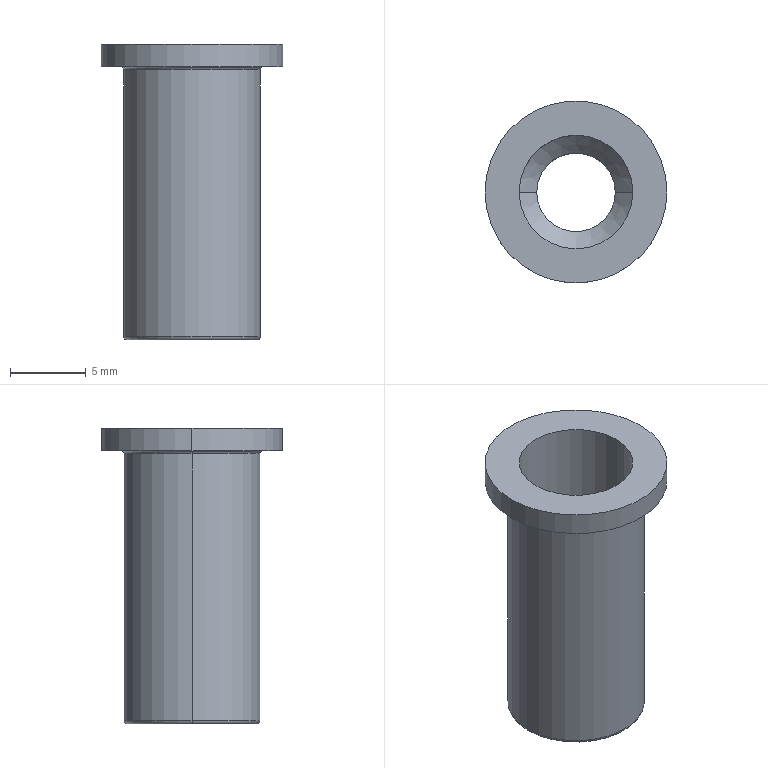Part | SolidWorks | features Chamfer 2, Cut 2, Boss 1, Extrusion 1, Fillet 1, LPattern 1, RevCut 1 | 1 solid | 19 faces | box 12 x 12 x 19.5 mm | volume 659.077 mm3 | cylinder 8 | cone 4 | torus 4 | plane 3 | commonest cylinder face diameters 5.188 x2 7.5 x2 9 x2 12 x2
STEP:
#1=CARTESIAN_POINT('',(2.594,0.,-19.241));
#2=VERTEX_POINT('',#1);
#3=CARTESIAN_POINT('',(-2.594,0.,-19.241));
#4=VERTEX_POINT('',#3);
#5=CARTESIAN_POINT('',(0.,0.,-19.241));
#6=DIRECTION('',(0.,0.,-1.));
#7=DIRECTION('',(-1.,0.,0.));
#8=AXIS2_PLACEMENT_3D('',#5,#6,#7);
#9=CIRCLE('',#8,2.594);
#10=EDGE_CURVE('',#2,#4,#9,.T.);
#11=ORIENTED_EDGE('',*,*,#10,.F.);
#12=CARTESIAN_POINT('',(2.853,0.,-19.5));
#13=VERTEX_POINT('',#12);
#14=CARTESIAN_POINT('',(2.853,0.,-19.5));
#15=DIRECTION('',(0.7071,0.,-0.7071));
#16=VECTOR('',#15,1000.);
#17=LINE('',#14,#16);
#18=EDGE_CURVE('',#2,#13,#17,.T.);
#19=ORIENTED_EDGE('',*,*,#18,.T.);
#20=CARTESIAN_POINT('',(-2.853,0.,-19.5));
#21=VERTEX_POINT('',#20);
#22=CARTESIAN_POINT('',(0.,0.,-19.5));
#23=DIRECTION('',(0.,0.,1.));
#24=DIRECTION('',(-1.,0.,0.));
#25=AXIS2_PLACEMENT_3D('',#22,#23,#24);
#26=CIRCLE('',#25,2.853);
#27=EDGE_CURVE('',#21,#13,#26,.T.);
#28=ORIENTED_EDGE('',*,*,#27,.F.);
#29=CARTESIAN_POINT('',(-2.853,0.,-19.5));
#30=DIRECTION('',(-0.7071,0.,-0.7071));
#31=VECTOR('',#30,1000.);
#32=LINE('',#29,#31);
#33=EDGE_CURVE('',#4,#21,#32,.T.);
#34=ORIENTED_EDGE('',*,*,#33,.F.);
#35=EDGE_LOOP('',(#11,#19,#28,#34));
#36=FACE_OUTER_BOUND('',#35,.T.);
#37=CARTESIAN_POINT('',(0.,0.,-19.5));
#38=DIRECTION('',(0.,0.,-1.));
#39=DIRECTION('',(-1.,0.,0.));
#40=AXIS2_PLACEMENT_3D('',#37,#38,#39);
#41=CONICAL_SURFACE('',#40,2.853,0.7854);
#42=ADVANCED_FACE('',(#36),#41,.F.);
#43=CARTESIAN_POINT('',(-2.594,0.,-11.156));
#44=VERTEX_POINT('',#43);
#45=CARTESIAN_POINT('',(2.594,0.,-11.156));
#46=VERTEX_POINT('',#45);
#47=CARTESIAN_POINT('',(0.,0.,-11.156));
#48=DIRECTION('',(0.,0.,1.));
#49=DIRECTION('',(1.,0.,0.));
#50=AXIS2_PLACEMENT_3D('',#47,#48,#49);
#51=CIRCLE('',#50,2.594);
#52=EDGE_CURVE('',#44,#46,#51,.T.);
#53=ORIENTED_EDGE('',*,*,#52,.F.);
#54=CARTESIAN_POINT('',(-3.75,0.,-10.));
#55=VERTEX_POINT('',#54);
#56=CARTESIAN_POINT('',(-2.594,0.,-11.156));
#57=DIRECTION('',(-0.7071,0.,0.7071));
#58=VECTOR('',#57,1000.);
#59=LINE('',#56,#58);
#60=EDGE_CURVE('',#44,#55,#59,.T.);
#61=ORIENTED_EDGE('',*,*,#60,.T.);
#62=CARTESIAN_POINT('',(3.75,0.,-10.));
#63=VERTEX_POINT('',#62);
#64=CARTESIAN_POINT('',(0.,0.,-10.));
#65=DIRECTION('',(0.,0.,1.));
#66=DIRECTION('',(1.,0.,0.));
#67=AXIS2_PLACEMENT_3D('',#64,#65,#66);
#68=CIRCLE('',#67,3.75);
#69=EDGE_CURVE('',#55,#63,#68,.T.);
#70=ORIENTED_EDGE('',*,*,#69,.T.);
#71=CARTESIAN_POINT('',(2.594,0.,-11.156));
#72=DIRECTION('',(0.7071,0.,0.7071));
#73=VECTOR('',#72,1000.);
#74=LINE('',#71,#73);
#75=EDGE_CURVE('',#46,#63,#74,.T.);
#76=ORIENTED_EDGE('',*,*,#75,.F.);
#77=EDGE_LOOP('',(#53,#61,#70,#76));
#78=FACE_OUTER_BOUND('',#77,.T.);
#79=CARTESIAN_POINT('',(0.,0.,-11.156));
#80=DIRECTION('',(0.,0.,1.));
#81=DIRECTION('',(1.,0.,0.));
#82=AXIS2_PLACEMENT_3D('',#79,#80,#81);
#83=CONICAL_SURFACE('',#82,2.594,0.7854);
#84=ADVANCED_FACE('',(#78),#83,.F.);
#85=CARTESIAN_POINT('',(-4.7,0.,-1.5));
#86=VERTEX_POINT('',#85);
#87=CARTESIAN_POINT('',(4.7,0.,-1.5));
#88=VERTEX_POINT('',#87);
#89=CARTESIAN_POINT('',(0.,0.,-1.5));
#90=DIRECTION('',(0.,0.,1.));
#91=DIRECTION('',(1.,0.,0.));
#92=AXIS2_PLACEMENT_3D('',#89,#90,#91);
#93=CIRCLE('',#92,4.7);
#94=EDGE_CURVE('',#86,#88,#93,.T.);
#95=ORIENTED_EDGE('',*,*,#94,.F.);
#96=CARTESIAN_POINT('',(-4.5,0.,-1.7));
#97=VERTEX_POINT('',#96);
#98=CARTESIAN_POINT('',(-4.7,0.,-1.7));
#99=DIRECTION('',(0.,1.,0.));
#100=DIRECTION('',(-1.,0.,0.));
#101=AXIS2_PLACEMENT_3D('',#98,#99,#100);
#102=CIRCLE('',#101,0.2);
#103=EDGE_CURVE('',#86,#97,#102,.T.);
#104=ORIENTED_EDGE('',*,*,#103,.T.);
#105=CARTESIAN_POINT('',(4.5,0.,-1.7));
#106=VERTEX_POINT('',#105);
#107=CARTESIAN_POINT('',(0.,0.,-1.7));
#108=DIRECTION('',(0.,0.,-1.));
#109=DIRECTION('',(1.,0.,0.));
#110=AXIS2_PLACEMENT_3D('',#107,#108,#109);
#111=CIRCLE('',#110,4.5);
#112=EDGE_CURVE('',#106,#97,#111,.T.);
#113=ORIENTED_EDGE('',*,*,#112,.F.);
#114=CARTESIAN_POINT('',(4.7,0.,-1.7));
#115=DIRECTION('',(0.,-1.,0.));
#116=DIRECTION('',(0.,0.,-1.));
#117=AXIS2_PLACEMENT_3D('',#114,#115,#116);
#118=CIRCLE('',#117,0.2);
#119=EDGE_CURVE('',#88,#106,#118,.T.);
#120=ORIENTED_EDGE('',*,*,#119,.F.);
#121=EDGE_LOOP('',(#95,#104,#113,#120));
#122=FACE_OUTER_BOUND('',#121,.T.);
#123=CARTESIAN_POINT('',(0.,0.,-1.7));
#124=DIRECTION('',(0.,0.,1.));
#125=DIRECTION('',(1.,0.,0.));
#126=AXIS2_PLACEMENT_3D('',#123,#124,#125);
#127=TOROIDAL_SURFACE('',#126,4.7,0.2);
#128=ADVANCED_FACE('',(#122),#127,.F.);
#129=CARTESIAN_POINT('',(4.5,0.,-19.3));
#130=VERTEX_POINT('',#129);
#131=CARTESIAN_POINT('',(-4.5,0.,-19.3));
#132=VERTEX_POINT('',#131);
#133=CARTESIAN_POINT('',(0.,0.,-19.3));
#134=DIRECTION('',(0.,0.,1.));
#135=DIRECTION('',(-1.,0.,0.));
#136=AXIS2_PLACEMENT_3D('',#133,#134,#135);
#137=CIRCLE('',#136,4.5);
#138=EDGE_CURVE('',#130,#132,#137,.T.);
#139=ORIENTED_EDGE('',*,*,#138,.F.);
#140=CARTESIAN_POINT('',(4.3,0.,-19.5));
#141=VERTEX_POINT('',#140);
#142=CARTESIAN_POINT('',(4.3,0.,-19.3));
#143=DIRECTION('',(0.,1.,0.));
#144=DIRECTION('',(-1.,0.,0.));
#145=AXIS2_PLACEMENT_3D('',#142,#143,#144);
#146=CIRCLE('',#145,0.2);
#147=EDGE_CURVE('',#130,#141,#146,.T.);
#148=ORIENTED_EDGE('',*,*,#147,.T.);
#149=CARTESIAN_POINT('',(-4.3,0.,-19.5));
#150=VERTEX_POINT('',#149);
#151=CARTESIAN_POINT('',(0.,0.,-19.5));
#152=DIRECTION('',(0.,0.,-1.));
#153=DIRECTION('',(-1.,0.,0.));
#154=AXIS2_PLACEMENT_3D('',#151,#152,#153);
#155=CIRCLE('',#154,4.3);
#156=EDGE_CURVE('',#150,#141,#155,.T.);
#157=ORIENTED_EDGE('',*,*,#156,.F.);
#158=CARTESIAN_POINT('',(-4.3,0.,-19.3));
#159=DIRECTION('',(0.,-1.,0.));
#160=DIRECTION('',(0.,0.,-1.));
#161=AXIS2_PLACEMENT_3D('',#158,#159,#160);
#162=CIRCLE('',#161,0.2);
#163=EDGE_CURVE('',#132,#150,#162,.T.);
#164=ORIENTED_EDGE('',*,*,#163,.F.);
#165=EDGE_LOOP('',(#139,#148,#157,#164));
#166=FACE_OUTER_BOUND('',#165,.T.);
#167=CARTESIAN_POINT('',(0.,0.,-19.3));
#168=DIRECTION('',(0.,0.,-1.));
#169=DIRECTION('',(-1.,0.,0.));
#170=AXIS2_PLACEMENT_3D('',#167,#168,#169);
#171=TOROIDAL_SURFACE('',#170,4.3,0.2);
#172=ADVANCED_FACE('',(#166),#171,.T.);
#173=ORIENTED_EDGE('',*,*,#10,.T.);
#174=CARTESIAN_POINT('',(-2.594,0.,-19.5));
#175=DIRECTION('',(0.,0.,1.));
#176=VECTOR('',#175,1000.);
#177=LINE('',#174,#176);
#178=EDGE_CURVE('',#4,#44,#177,.T.);
#179=ORIENTED_EDGE('',*,*,#178,.T.);
#180=ORIENTED_EDGE('',*,*,#52,.T.);
#181=CARTESIAN_POINT('',(2.594,0.,-19.5));
#182=DIRECTION('',(0.,0.,1.));
#183=VECTOR('',#182,1000.);
#184=LINE('',#181,#183);
#185=EDGE_CURVE('',#2,#46,#184,.T.);
#186=ORIENTED_EDGE('',*,*,#185,.F.);
#187=EDGE_LOOP('',(#173,#179,#180,#186));
#188=FACE_OUTER_BOUND('',#187,.T.);
#189=CARTESIAN_POINT('',(0.,0.,-19.5));
#190=DIRECTION('',(0.,0.,1.));
#191=DIRECTION('',(1.,0.,0.));
#192=AXIS2_PLACEMENT_3D('',#189,#190,#191);
#193=CYLINDRICAL_SURFACE('',#192,2.594);
#194=ADVANCED_FACE('',(#188),#193,.F.);
#195=ORIENTED_EDGE('',*,*,#69,.F.);
#196=CARTESIAN_POINT('',(-3.75,0.,0.));
#197=VERTEX_POINT('',#196);
#198=CARTESIAN_POINT('',(-3.75,0.,-10.));
#199=DIRECTION('',(0.,0.,1.));
#200=VECTOR('',#199,1000.);
#201=LINE('',#198,#200);
#202=EDGE_CURVE('',#55,#197,#201,.T.);
#203=ORIENTED_EDGE('',*,*,#202,.T.);
#204=CARTESIAN_POINT('',(3.75,0.,0.));
#205=VERTEX_POINT('',#204);
#206=CARTESIAN_POINT('',(0.,0.,0.));
#207=DIRECTION('',(0.,0.,1.));
#208=DIRECTION('',(1.,0.,0.));
#209=AXIS2_PLACEMENT_3D('',#206,#207,#208);
#210=CIRCLE('',#209,3.75);
#211=EDGE_CURVE('',#197,#205,#210,.T.);
#212=ORIENTED_EDGE('',*,*,#211,.T.);
#213=CARTESIAN_POINT('',(3.75,0.,-10.));
#214=DIRECTION('',(0.,0.,1.));
#215=VECTOR('',#214,1000.);
#216=LINE('',#213,#215);
#217=EDGE_CURVE('',#63,#205,#216,.T.);
#218=ORIENTED_EDGE('',*,*,#217,.F.);
#219=EDGE_LOOP('',(#195,#203,#212,#218));
#220=FACE_OUTER_BOUND('',#219,.T.);
#221=CARTESIAN_POINT('',(0.,0.,-10.));
#222=DIRECTION('',(0.,0.,1.));
#223=DIRECTION('',(1.,0.,0.));
#224=AXIS2_PLACEMENT_3D('',#221,#222,#223);
#225=CYLINDRICAL_SURFACE('',#224,3.75);
#226=ADVANCED_FACE('',(#220),#225,.F.);
#227=ORIENTED_EDGE('',*,*,#138,.T.);
#228=CARTESIAN_POINT('',(-4.5,0.,-19.5));
#229=DIRECTION('',(0.,0.,1.));
#230=VECTOR('',#229,1000.);
#231=LINE('',#228,#230);
#232=EDGE_CURVE('',#132,#97,#231,.T.);
#233=ORIENTED_EDGE('',*,*,#232,.T.);
#234=CARTESIAN_POINT('',(0.,0.,-1.7));
#235=DIRECTION('',(0.,0.,-1.));
#236=DIRECTION('',(1.,0.,0.));
#237=AXIS2_PLACEMENT_3D('',#234,#235,#236);
#238=CIRCLE('',#237,4.5);
#239=EDGE_CURVE('',#97,#106,#238,.T.);
#240=ORIENTED_EDGE('',*,*,#239,.T.);
#241=CARTESIAN_POINT('',(4.5,0.,-19.5));
#242=DIRECTION('',(0.,0.,1.));
#243=VECTOR('',#242,1000.);
#244=LINE('',#241,#243);
#245=EDGE_CURVE('',#130,#106,#244,.T.);
#246=ORIENTED_EDGE('',*,*,#245,.F.);
#247=EDGE_LOOP('',(#227,#233,#240,#246));
#248=FACE_OUTER_BOUND('',#247,.T.);
#249=CARTESIAN_POINT('',(0.,0.,-19.5));
#250=DIRECTION('',(0.,0.,1.));
#251=DIRECTION('',(1.,0.,0.));
#252=AXIS2_PLACEMENT_3D('',#249,#250,#251);
#253=CYLINDRICAL_SURFACE('',#252,4.5);
#254=ADVANCED_FACE('',(#248),#253,.T.);
#255=CARTESIAN_POINT('',(6.,0.,-1.5));
#256=VERTEX_POINT('',#255);
#257=CARTESIAN_POINT('',(-6.,0.,-1.5));
#258=VERTEX_POINT('',#257);
#259=CARTESIAN_POINT('',(0.,0.,-1.5));
#260=DIRECTION('',(0.,0.,1.));
#261=DIRECTION('',(1.,0.,0.));
#262=AXIS2_PLACEMENT_3D('',#259,#260,#261);
#263=CIRCLE('',#262,6.);
#264=EDGE_CURVE('',#256,#258,#263,.T.);
#265=ORIENTED_EDGE('',*,*,#264,.T.);
#266=CARTESIAN_POINT('',(-6.,0.,0.));
#267=VERTEX_POINT('',#266);
#268=CARTESIAN_POINT('',(-6.,0.,-1.5));
#269=DIRECTION('',(0.,0.,1.));
#270=VECTOR('',#269,1000.);
#271=LINE('',#268,#270);
#272=EDGE_CURVE('',#258,#267,#271,.T.);
#273=ORIENTED_EDGE('',*,*,#272,.T.);
#274=CARTESIAN_POINT('',(6.,0.,0.));
#275=VERTEX_POINT('',#274);
#276=CARTESIAN_POINT('',(0.,0.,0.));
#277=DIRECTION('',(0.,0.,1.));
#278=DIRECTION('',(1.,0.,0.));
#279=AXIS2_PLACEMENT_3D('',#276,#277,#278);
#280=CIRCLE('',#279,6.);
#281=EDGE_CURVE('',#275,#267,#280,.T.);
#282=ORIENTED_EDGE('',*,*,#281,.F.);
#283=CARTESIAN_POINT('',(6.,0.,-1.5));
#284=DIRECTION('',(0.,0.,1.));
#285=VECTOR('',#284,1000.);
#286=LINE('',#283,#285);
#287=EDGE_CURVE('',#256,#275,#286,.T.);
#288=ORIENTED_EDGE('',*,*,#287,.F.);
#289=EDGE_LOOP('',(#265,#273,#282,#288));
#290=FACE_OUTER_BOUND('',#289,.T.);
#291=CARTESIAN_POINT('',(0.,0.,-1.5));
#292=DIRECTION('',(0.,0.,1.));
#293=DIRECTION('',(1.,0.,0.));
#294=AXIS2_PLACEMENT_3D('',#291,#292,#293);
#295=CYLINDRICAL_SURFACE('',#294,6.);
#296=ADVANCED_FACE('',(#290),#295,.T.);
#297=CARTESIAN_POINT('',(0.,0.,-1.5));
#298=DIRECTION('',(0.,0.,1.));
#299=DIRECTION('',(1.,0.,0.));
#300=AXIS2_PLACEMENT_3D('',#297,#298,#299);
#301=CIRCLE('',#300,4.7);
#302=EDGE_CURVE('',#88,#86,#301,.T.);
#303=ORIENTED_EDGE('',*,*,#302,.T.);
#304=ORIENTED_EDGE('',*,*,#94,.T.);
#305=EDGE_LOOP('',(#303,#304));
#306=FACE_BOUND('',#305,.T.);
#307=ORIENTED_EDGE('',*,*,#264,.F.);
#308=CARTESIAN_POINT('',(0.,0.,-1.5));
#309=DIRECTION('',(0.,0.,1.));
#310=DIRECTION('',(1.,0.,0.));
#311=AXIS2_PLACEMENT_3D('',#308,#309,#310);
#312=CIRCLE('',#311,6.);
#313=EDGE_CURVE('',#258,#256,#312,.T.);
#314=ORIENTED_EDGE('',*,*,#313,.F.);
#315=EDGE_LOOP('',(#307,#314));
#316=FACE_OUTER_BOUND('',#315,.T.);
#317=CARTESIAN_POINT('',(0.,0.,-1.5));
#318=DIRECTION('',(0.,0.,1.));
#319=DIRECTION('',(1.,0.,0.));
#320=AXIS2_PLACEMENT_3D('',#317,#318,#319);
#321=PLANE('',#320);
#322=ADVANCED_FACE('',(#306,#316),#321,.F.);
#323=ORIENTED_EDGE('',*,*,#272,.F.);
#324=ORIENTED_EDGE('',*,*,#313,.T.);
#325=ORIENTED_EDGE('',*,*,#287,.T.);
#326=CARTESIAN_POINT('',(0.,0.,0.));
#327=DIRECTION('',(0.,0.,1.));
#328=DIRECTION('',(1.,0.,0.));
#329=AXIS2_PLACEMENT_3D('',#326,#327,#328);
#330=CIRCLE('',#329,6.);
#331=EDGE_CURVE('',#267,#275,#330,.T.);
#332=ORIENTED_EDGE('',*,*,#331,.F.);
#333=EDGE_LOOP('',(#323,#324,#325,#332));
#334=FACE_OUTER_BOUND('',#333,.T.);
#335=CARTESIAN_POINT('',(0.,0.,-1.5));
#336=DIRECTION('',(0.,0.,1.));
#337=DIRECTION('',(1.,0.,0.));
#338=AXIS2_PLACEMENT_3D('',#335,#336,#337);
#339=CYLINDRICAL_SURFACE('',#338,6.);
#340=ADVANCED_FACE('',(#334),#339,.T.);
#341=CARTESIAN_POINT('',(0.,0.,0.));
#342=DIRECTION('',(0.,0.,1.));
#343=DIRECTION('',(1.,0.,0.));
#344=AXIS2_PLACEMENT_3D('',#341,#342,#343);
#345=CIRCLE('',#344,3.75);
#346=EDGE_CURVE('',#205,#197,#345,.T.);
#347=ORIENTED_EDGE('',*,*,#346,.F.);
#348=ORIENTED_EDGE('',*,*,#211,.F.);
#349=EDGE_LOOP('',(#347,#348));
#350=FACE_BOUND('',#349,.T.);
#351=ORIENTED_EDGE('',*,*,#281,.T.);
#352=ORIENTED_EDGE('',*,*,#331,.T.);
#353=EDGE_LOOP('',(#351,#352));
#354=FACE_OUTER_BOUND('',#353,.T.);
#355=CARTESIAN_POINT('',(0.,0.,0.));
#356=DIRECTION('',(0.,0.,1.));
#357=DIRECTION('',(1.,0.,0.));
#358=AXIS2_PLACEMENT_3D('',#355,#356,#357);
#359=PLANE('',#358);
#360=ADVANCED_FACE('',(#350,#354),#359,.T.);
#361=ORIENTED_EDGE('',*,*,#232,.F.);
#362=CARTESIAN_POINT('',(0.,0.,-19.3));
#363=DIRECTION('',(0.,0.,1.));
#364=DIRECTION('',(-1.,0.,0.));
#365=AXIS2_PLACEMENT_3D('',#362,#363,#364);
#366=CIRCLE('',#365,4.5);
#367=EDGE_CURVE('',#132,#130,#366,.T.);
#368=ORIENTED_EDGE('',*,*,#367,.T.);
#369=ORIENTED_EDGE('',*,*,#245,.T.);
#370=ORIENTED_EDGE('',*,*,#112,.T.);
#371=EDGE_LOOP('',(#361,#368,#369,#370));
#372=FACE_OUTER_BOUND('',#371,.T.);
#373=CARTESIAN_POINT('',(0.,0.,-19.5));
#374=DIRECTION('',(0.,0.,1.));
#375=DIRECTION('',(1.,0.,0.));
#376=AXIS2_PLACEMENT_3D('',#373,#374,#375);
#377=CYLINDRICAL_SURFACE('',#376,4.5);
#378=ADVANCED_FACE('',(#372),#377,.T.);
#379=ORIENTED_EDGE('',*,*,#27,.T.);
#380=CARTESIAN_POINT('',(0.,0.,-19.5));
#381=DIRECTION('',(0.,0.,1.));
#382=DIRECTION('',(-1.,0.,0.));
#383=AXIS2_PLACEMENT_3D('',#380,#381,#382);
#384=CIRCLE('',#383,2.853);
#385=EDGE_CURVE('',#13,#21,#384,.T.);
#386=ORIENTED_EDGE('',*,*,#385,.T.);
#387=EDGE_LOOP('',(#379,#386));
#388=FACE_BOUND('',#387,.T.);
#389=ORIENTED_EDGE('',*,*,#156,.T.);
#390=CARTESIAN_POINT('',(0.,0.,-19.5));
#391=DIRECTION('',(0.,0.,-1.));
#392=DIRECTION('',(-1.,0.,0.));
#393=AXIS2_PLACEMENT_3D('',#390,#391,#392);
#394=CIRCLE('',#393,4.3);
#395=EDGE_CURVE('',#141,#150,#394,.T.);
#396=ORIENTED_EDGE('',*,*,#395,.T.);
#397=EDGE_LOOP('',(#389,#396));
#398=FACE_OUTER_BOUND('',#397,.T.);
#399=CARTESIAN_POINT('',(0.,0.,-19.5));
#400=DIRECTION('',(0.,0.,-1.));
#401=DIRECTION('',(-1.,0.,0.));
#402=AXIS2_PLACEMENT_3D('',#399,#400,#401);
#403=PLANE('',#402);
#404=ADVANCED_FACE('',(#388,#398),#403,.T.);
#405=ORIENTED_EDGE('',*,*,#202,.F.);
#406=CARTESIAN_POINT('',(0.,0.,-10.));
#407=DIRECTION('',(0.,0.,1.));
#408=DIRECTION('',(1.,0.,0.));
#409=AXIS2_PLACEMENT_3D('',#406,#407,#408);
#410=CIRCLE('',#409,3.75);
#411=EDGE_CURVE('',#63,#55,#410,.T.);
#412=ORIENTED_EDGE('',*,*,#411,.F.);
#413=ORIENTED_EDGE('',*,*,#217,.T.);
#414=ORIENTED_EDGE('',*,*,#346,.T.);
#415=EDGE_LOOP('',(#405,#412,#413,#414));
#416=FACE_OUTER_BOUND('',#415,.T.);
#417=CARTESIAN_POINT('',(0.,0.,-10.));
#418=DIRECTION('',(0.,0.,1.));
#419=DIRECTION('',(1.,0.,0.));
#420=AXIS2_PLACEMENT_3D('',#417,#418,#419);
#421=CYLINDRICAL_SURFACE('',#420,3.75);
#422=ADVANCED_FACE('',(#416),#421,.F.);
#423=ORIENTED_EDGE('',*,*,#178,.F.);
#424=CARTESIAN_POINT('',(0.,0.,-19.241));
#425=DIRECTION('',(0.,0.,-1.));
#426=DIRECTION('',(-1.,0.,0.));
#427=AXIS2_PLACEMENT_3D('',#424,#425,#426);
#428=CIRCLE('',#427,2.594);
#429=EDGE_CURVE('',#4,#2,#428,.T.);
#430=ORIENTED_EDGE('',*,*,#429,.T.);
#431=ORIENTED_EDGE('',*,*,#185,.T.);
#432=CARTESIAN_POINT('',(0.,0.,-11.156));
#433=DIRECTION('',(0.,0.,1.));
#434=DIRECTION('',(1.,0.,0.));
#435=AXIS2_PLACEMENT_3D('',#432,#433,#434);
#436=CIRCLE('',#435,2.594);
#437=EDGE_CURVE('',#46,#44,#436,.T.);
#438=ORIENTED_EDGE('',*,*,#437,.T.);
#439=EDGE_LOOP('',(#423,#430,#431,#438));
#440=FACE_OUTER_BOUND('',#439,.T.);
#441=CARTESIAN_POINT('',(0.,0.,-19.5));
#442=DIRECTION('',(0.,0.,1.));
#443=DIRECTION('',(1.,0.,0.));
#444=AXIS2_PLACEMENT_3D('',#441,#442,#443);
#445=CYLINDRICAL_SURFACE('',#444,2.594);
#446=ADVANCED_FACE('',(#440),#445,.F.);
#447=ORIENTED_EDGE('',*,*,#147,.F.);
#448=ORIENTED_EDGE('',*,*,#367,.F.);
#449=ORIENTED_EDGE('',*,*,#163,.T.);
#450=ORIENTED_EDGE('',*,*,#395,.F.);
#451=EDGE_LOOP('',(#447,#448,#449,#450));
#452=FACE_OUTER_BOUND('',#451,.T.);
#453=CARTESIAN_POINT('',(0.,0.,-19.3));
#454=DIRECTION('',(0.,0.,-1.));
#455=DIRECTION('',(-1.,0.,0.));
#456=AXIS2_PLACEMENT_3D('',#453,#454,#455);
#457=TOROIDAL_SURFACE('',#456,4.3,0.2);
#458=ADVANCED_FACE('',(#452),#457,.T.);
#459=ORIENTED_EDGE('',*,*,#103,.F.);
#460=ORIENTED_EDGE('',*,*,#302,.F.);
#461=ORIENTED_EDGE('',*,*,#119,.T.);
#462=ORIENTED_EDGE('',*,*,#239,.F.);
#463=EDGE_LOOP('',(#459,#460,#461,#462));
#464=FACE_OUTER_BOUND('',#463,.T.);
#465=CARTESIAN_POINT('',(0.,0.,-1.7));
#466=DIRECTION('',(0.,0.,1.));
#467=DIRECTION('',(1.,0.,0.));
#468=AXIS2_PLACEMENT_3D('',#465,#466,#467);
#469=TOROIDAL_SURFACE('',#468,4.7,0.2);
#470=ADVANCED_FACE('',(#464),#469,.F.);
#471=ORIENTED_EDGE('',*,*,#60,.F.);
#472=ORIENTED_EDGE('',*,*,#437,.F.);
#473=ORIENTED_EDGE('',*,*,#75,.T.);
#474=ORIENTED_EDGE('',*,*,#411,.T.);
#475=EDGE_LOOP('',(#471,#472,#473,#474));
#476=FACE_OUTER_BOUND('',#475,.T.);
#477=CARTESIAN_POINT('',(0.,0.,-11.156));
#478=DIRECTION('',(0.,0.,1.));
#479=DIRECTION('',(1.,0.,0.));
#480=AXIS2_PLACEMENT_3D('',#477,#478,#479);
#481=CONICAL_SURFACE('',#480,2.594,0.7854);
#482=ADVANCED_FACE('',(#476),#481,.F.);
#483=ORIENTED_EDGE('',*,*,#18,.F.);
#484=ORIENTED_EDGE('',*,*,#429,.F.);
#485=ORIENTED_EDGE('',*,*,#33,.T.);
#486=ORIENTED_EDGE('',*,*,#385,.F.);
#487=EDGE_LOOP('',(#483,#484,#485,#486));
#488=FACE_OUTER_BOUND('',#487,.T.);
#489=CARTESIAN_POINT('',(0.,0.,-19.5));
#490=DIRECTION('',(0.,0.,-1.));
#491=DIRECTION('',(-1.,0.,0.));
#492=AXIS2_PLACEMENT_3D('',#489,#490,#491);
#493=CONICAL_SURFACE('',#492,2.853,0.7854);
#494=ADVANCED_FACE('',(#488),#493,.F.);
#495=CLOSED_SHELL('',(#42,#84,#128,#172,#194,#226,#254,#296,#322,#340,#360,#378,#404,#422,#446,#458,#470,#482,#494));
#496=MANIFOLD_SOLID_BREP('',#495);
#497=CARTESIAN_POINT('',(0.,0.,0.));
#498=DIRECTION('',(0.,0.,1.));
#499=DIRECTION('',(1.,0.,0.));
#500=AXIS2_PLACEMENT_3D('',#497,#498,#499);
#501=(LENGTH_UNIT()NAMED_UNIT(*)SI_UNIT(.MILLI.,.METRE.));
#502=UNCERTAINTY_MEASURE_WITH_UNIT(LENGTH_MEASURE(0.00001),#501,'','');
#503=(NAMED_UNIT(*)PLANE_ANGLE_UNIT()SI_UNIT($,.RADIAN.));
#504=(NAMED_UNIT(*)SI_UNIT($,.STERADIAN.)SOLID_ANGLE_UNIT());
#505=(GEOMETRIC_REPRESENTATION_CONTEXT(3)GLOBAL_UNCERTAINTY_ASSIGNED_CONTEXT((#502))GLOBAL_UNIT_ASSIGNED_CONTEXT((#501,#503,#504))REPRESENTATION_CONTEXT('',''));
#506=ADVANCED_BREP_SHAPE_REPRESENTATION('',(#496,#500),#505);